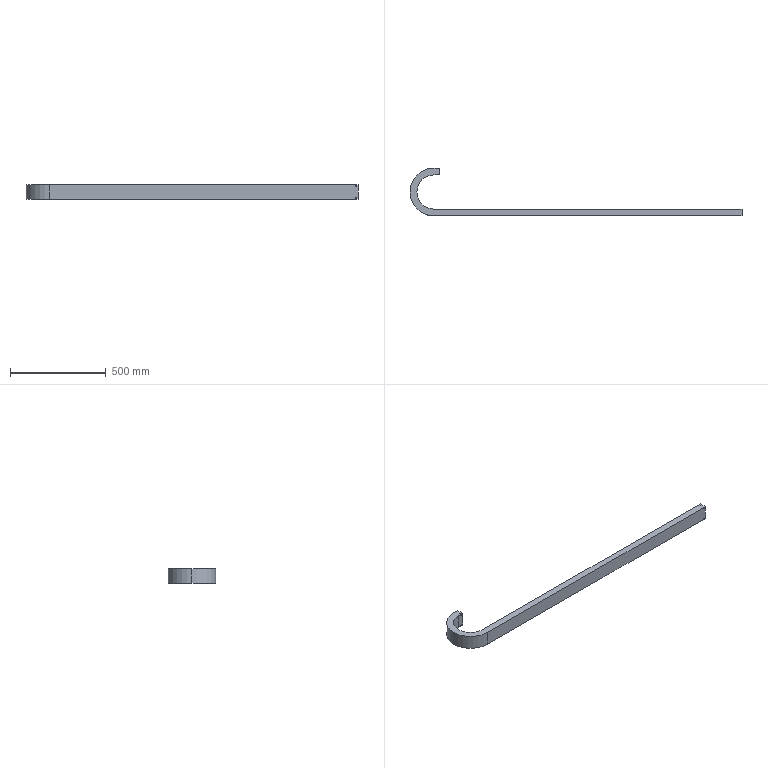Part | STEP file | 1 solid | 20 faces | box 1732 x 250 x 75 mm | volume 5324161 mm3 | cylinder 12 | plane 8 | commonest cylinder face diameters 4.2 x8 178 x2 250 x2